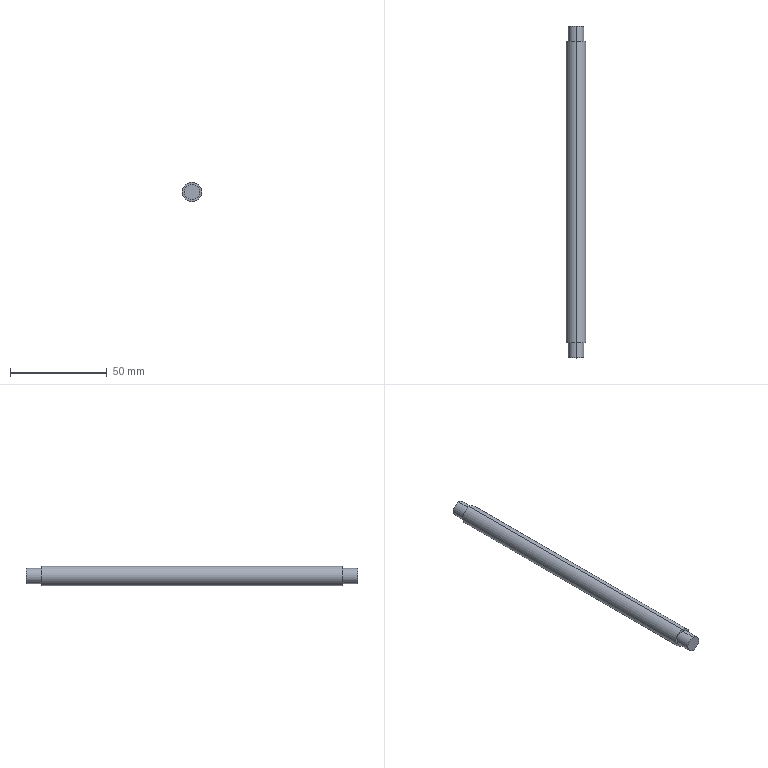Part | SolidWorks | features Extrusion 1, ICE 1, MirrorPattern 1 | 1 solid | 10 faces | box 10 x 172 x 10 mm | volume 13056 mm3 | cylinder 6 | plane 4 | commonest cylinder face diameters 8 x4 10 x2
STEP:
#1=CARTESIAN_POINT('',(0.,-3.386,0.1575));
#2=VERTEX_POINT('',#1);
#3=CARTESIAN_POINT('',(0.,-3.386,-0.1575));
#4=VERTEX_POINT('',#3);
#5=CARTESIAN_POINT('',(0.,-3.386,0.));
#6=DIRECTION('',(0.,1.,0.));
#7=DIRECTION('',(0.,0.,1.));
#8=AXIS2_PLACEMENT_3D('',#5,#6,#7);
#9=CIRCLE('',#8,0.1575);
#10=EDGE_CURVE('',#2,#4,#9,.T.);
#11=ORIENTED_EDGE('',*,*,#10,.T.);
#12=CARTESIAN_POINT('',(0.,-3.071,-0.1575));
#13=VERTEX_POINT('',#12);
#14=CARTESIAN_POINT('',(0.,-3.386,-0.1575));
#15=DIRECTION('',(0.,1.,0.));
#16=VECTOR('',#15,39.37);
#17=LINE('',#14,#16);
#18=EDGE_CURVE('',#4,#13,#17,.T.);
#19=ORIENTED_EDGE('',*,*,#18,.T.);
#20=CARTESIAN_POINT('',(0.,-3.071,0.1575));
#21=VERTEX_POINT('',#20);
#22=CARTESIAN_POINT('',(0.,-3.071,0.));
#23=DIRECTION('',(0.,1.,0.));
#24=DIRECTION('',(0.,0.,1.));
#25=AXIS2_PLACEMENT_3D('',#22,#23,#24);
#26=CIRCLE('',#25,0.1575);
#27=EDGE_CURVE('',#21,#13,#26,.T.);
#28=ORIENTED_EDGE('',*,*,#27,.F.);
#29=CARTESIAN_POINT('',(0.,-3.386,0.1575));
#30=DIRECTION('',(0.,1.,0.));
#31=VECTOR('',#30,39.37);
#32=LINE('',#29,#31);
#33=EDGE_CURVE('',#2,#21,#32,.T.);
#34=ORIENTED_EDGE('',*,*,#33,.F.);
#35=EDGE_LOOP('',(#11,#19,#28,#34));
#36=FACE_OUTER_BOUND('',#35,.T.);
#37=CARTESIAN_POINT('',(0.,-3.386,0.));
#38=DIRECTION('',(0.,1.,0.));
#39=DIRECTION('',(0.,0.,1.));
#40=AXIS2_PLACEMENT_3D('',#37,#38,#39);
#41=CYLINDRICAL_SURFACE('',#40,0.1575);
#42=ADVANCED_FACE('',(#36),#41,.T.);
#43=CARTESIAN_POINT('',(0.,3.386,0.1575));
#44=VERTEX_POINT('',#43);
#45=CARTESIAN_POINT('',(0.,3.386,-0.1575));
#46=VERTEX_POINT('',#45);
#47=CARTESIAN_POINT('',(0.,3.386,0.));
#48=DIRECTION('',(0.,1.,0.));
#49=DIRECTION('',(0.,0.,1.));
#50=AXIS2_PLACEMENT_3D('',#47,#48,#49);
#51=CIRCLE('',#50,0.1575);
#52=EDGE_CURVE('',#44,#46,#51,.T.);
#53=ORIENTED_EDGE('',*,*,#52,.F.);
#54=CARTESIAN_POINT('',(0.,3.071,0.1575));
#55=VERTEX_POINT('',#54);
#56=CARTESIAN_POINT('',(0.,3.386,0.1575));
#57=DIRECTION('',(0.,-1.,0.));
#58=VECTOR('',#57,39.37);
#59=LINE('',#56,#58);
#60=EDGE_CURVE('',#44,#55,#59,.T.);
#61=ORIENTED_EDGE('',*,*,#60,.T.);
#62=CARTESIAN_POINT('',(0.,3.071,-0.1575));
#63=VERTEX_POINT('',#62);
#64=CARTESIAN_POINT('',(0.,3.071,0.));
#65=DIRECTION('',(0.,1.,0.));
#66=DIRECTION('',(0.,0.,1.));
#67=AXIS2_PLACEMENT_3D('',#64,#65,#66);
#68=CIRCLE('',#67,0.1575);
#69=EDGE_CURVE('',#55,#63,#68,.T.);
#70=ORIENTED_EDGE('',*,*,#69,.T.);
#71=CARTESIAN_POINT('',(0.,3.386,-0.1575));
#72=DIRECTION('',(0.,-1.,0.));
#73=VECTOR('',#72,39.37);
#74=LINE('',#71,#73);
#75=EDGE_CURVE('',#46,#63,#74,.T.);
#76=ORIENTED_EDGE('',*,*,#75,.F.);
#77=EDGE_LOOP('',(#53,#61,#70,#76));
#78=FACE_OUTER_BOUND('',#77,.T.);
#79=CARTESIAN_POINT('',(0.,3.386,0.));
#80=DIRECTION('',(0.,-1.,0.));
#81=DIRECTION('',(0.,0.,-1.));
#82=AXIS2_PLACEMENT_3D('',#79,#80,#81);
#83=CYLINDRICAL_SURFACE('',#82,0.1575);
#84=ADVANCED_FACE('',(#78),#83,.T.);
#85=CARTESIAN_POINT('',(0.,3.071,0.1969));
#86=VERTEX_POINT('',#85);
#87=CARTESIAN_POINT('',(0.,3.071,-0.1969));
#88=VERTEX_POINT('',#87);
#89=CARTESIAN_POINT('',(0.,3.071,0.));
#90=DIRECTION('',(0.,1.,0.));
#91=DIRECTION('',(0.,0.,1.));
#92=AXIS2_PLACEMENT_3D('',#89,#90,#91);
#93=CIRCLE('',#92,0.1969);
#94=EDGE_CURVE('',#86,#88,#93,.T.);
#95=ORIENTED_EDGE('',*,*,#94,.F.);
#96=CARTESIAN_POINT('',(0.,-3.071,0.1969));
#97=VERTEX_POINT('',#96);
#98=CARTESIAN_POINT('',(0.,3.071,0.1969));
#99=DIRECTION('',(0.,-1.,0.));
#100=VECTOR('',#99,39.37);
#101=LINE('',#98,#100);
#102=EDGE_CURVE('',#86,#97,#101,.T.);
#103=ORIENTED_EDGE('',*,*,#102,.T.);
#104=CARTESIAN_POINT('',(0.,-3.071,-0.1969));
#105=VERTEX_POINT('',#104);
#106=CARTESIAN_POINT('',(0.,-3.071,0.));
#107=DIRECTION('',(0.,1.,0.));
#108=DIRECTION('',(0.,0.,1.));
#109=AXIS2_PLACEMENT_3D('',#106,#107,#108);
#110=CIRCLE('',#109,0.1969);
#111=EDGE_CURVE('',#97,#105,#110,.T.);
#112=ORIENTED_EDGE('',*,*,#111,.T.);
#113=CARTESIAN_POINT('',(0.,3.071,-0.1969));
#114=DIRECTION('',(0.,-1.,0.));
#115=VECTOR('',#114,39.37);
#116=LINE('',#113,#115);
#117=EDGE_CURVE('',#88,#105,#116,.T.);
#118=ORIENTED_EDGE('',*,*,#117,.F.);
#119=EDGE_LOOP('',(#95,#103,#112,#118));
#120=FACE_OUTER_BOUND('',#119,.T.);
#121=CARTESIAN_POINT('',(0.,3.071,0.));
#122=DIRECTION('',(0.,-1.,0.));
#123=DIRECTION('',(0.,0.,-1.));
#124=AXIS2_PLACEMENT_3D('',#121,#122,#123);
#125=CYLINDRICAL_SURFACE('',#124,0.1969);
#126=ADVANCED_FACE('',(#120),#125,.T.);
#127=ORIENTED_EDGE('',*,*,#102,.F.);
#128=CARTESIAN_POINT('',(0.,3.071,0.));
#129=DIRECTION('',(0.,1.,0.));
#130=DIRECTION('',(0.,0.,1.));
#131=AXIS2_PLACEMENT_3D('',#128,#129,#130);
#132=CIRCLE('',#131,0.1969);
#133=EDGE_CURVE('',#88,#86,#132,.T.);
#134=ORIENTED_EDGE('',*,*,#133,.F.);
#135=ORIENTED_EDGE('',*,*,#117,.T.);
#136=CARTESIAN_POINT('',(0.,-3.071,0.));
#137=DIRECTION('',(0.,1.,0.));
#138=DIRECTION('',(0.,0.,1.));
#139=AXIS2_PLACEMENT_3D('',#136,#137,#138);
#140=CIRCLE('',#139,0.1969);
#141=EDGE_CURVE('',#105,#97,#140,.T.);
#142=ORIENTED_EDGE('',*,*,#141,.T.);
#143=EDGE_LOOP('',(#127,#134,#135,#142));
#144=FACE_OUTER_BOUND('',#143,.T.);
#145=CARTESIAN_POINT('',(0.,3.071,0.));
#146=DIRECTION('',(0.,-1.,0.));
#147=DIRECTION('',(0.,0.,-1.));
#148=AXIS2_PLACEMENT_3D('',#145,#146,#147);
#149=CYLINDRICAL_SURFACE('',#148,0.1969);
#150=ADVANCED_FACE('',(#144),#149,.T.);
#151=CARTESIAN_POINT('',(0.,3.071,0.));
#152=DIRECTION('',(0.,1.,0.));
#153=DIRECTION('',(0.,0.,1.));
#154=AXIS2_PLACEMENT_3D('',#151,#152,#153);
#155=CIRCLE('',#154,0.1575);
#156=EDGE_CURVE('',#63,#55,#155,.T.);
#157=ORIENTED_EDGE('',*,*,#156,.F.);
#158=ORIENTED_EDGE('',*,*,#69,.F.);
#159=EDGE_LOOP('',(#157,#158));
#160=FACE_BOUND('',#159,.T.);
#161=ORIENTED_EDGE('',*,*,#133,.T.);
#162=ORIENTED_EDGE('',*,*,#94,.T.);
#163=EDGE_LOOP('',(#161,#162));
#164=FACE_OUTER_BOUND('',#163,.T.);
#165=CARTESIAN_POINT('',(0.,3.071,0.));
#166=DIRECTION('',(0.,1.,0.));
#167=DIRECTION('',(0.,0.,1.));
#168=AXIS2_PLACEMENT_3D('',#165,#166,#167);
#169=PLANE('',#168);
#170=ADVANCED_FACE('',(#160,#164),#169,.T.);
#171=ORIENTED_EDGE('',*,*,#27,.T.);
#172=CARTESIAN_POINT('',(0.,-3.071,0.));
#173=DIRECTION('',(0.,1.,0.));
#174=DIRECTION('',(0.,0.,1.));
#175=AXIS2_PLACEMENT_3D('',#172,#173,#174);
#176=CIRCLE('',#175,0.1575);
#177=EDGE_CURVE('',#13,#21,#176,.T.);
#178=ORIENTED_EDGE('',*,*,#177,.T.);
#179=EDGE_LOOP('',(#171,#178));
#180=FACE_BOUND('',#179,.T.);
#181=ORIENTED_EDGE('',*,*,#141,.F.);
#182=ORIENTED_EDGE('',*,*,#111,.F.);
#183=EDGE_LOOP('',(#181,#182));
#184=FACE_OUTER_BOUND('',#183,.T.);
#185=CARTESIAN_POINT('',(0.,-3.071,0.));
#186=DIRECTION('',(0.,1.,0.));
#187=DIRECTION('',(0.,0.,1.));
#188=AXIS2_PLACEMENT_3D('',#185,#186,#187);
#189=PLANE('',#188);
#190=ADVANCED_FACE('',(#180,#184),#189,.F.);
#191=ORIENTED_EDGE('',*,*,#60,.F.);
#192=CARTESIAN_POINT('',(0.,3.386,0.));
#193=DIRECTION('',(0.,1.,0.));
#194=DIRECTION('',(0.,0.,1.));
#195=AXIS2_PLACEMENT_3D('',#192,#193,#194);
#196=CIRCLE('',#195,0.1575);
#197=EDGE_CURVE('',#46,#44,#196,.T.);
#198=ORIENTED_EDGE('',*,*,#197,.F.);
#199=ORIENTED_EDGE('',*,*,#75,.T.);
#200=ORIENTED_EDGE('',*,*,#156,.T.);
#201=EDGE_LOOP('',(#191,#198,#199,#200));
#202=FACE_OUTER_BOUND('',#201,.T.);
#203=CARTESIAN_POINT('',(0.,3.386,0.));
#204=DIRECTION('',(0.,-1.,0.));
#205=DIRECTION('',(0.,0.,-1.));
#206=AXIS2_PLACEMENT_3D('',#203,#204,#205);
#207=CYLINDRICAL_SURFACE('',#206,0.1575);
#208=ADVANCED_FACE('',(#202),#207,.T.);
#209=ORIENTED_EDGE('',*,*,#197,.T.);
#210=ORIENTED_EDGE('',*,*,#52,.T.);
#211=EDGE_LOOP('',(#209,#210));
#212=FACE_OUTER_BOUND('',#211,.T.);
#213=CARTESIAN_POINT('',(0.,3.386,0.));
#214=DIRECTION('',(0.,1.,0.));
#215=DIRECTION('',(0.,0.,1.));
#216=AXIS2_PLACEMENT_3D('',#213,#214,#215);
#217=PLANE('',#216);
#218=ADVANCED_FACE('',(#212),#217,.T.);
#219=ORIENTED_EDGE('',*,*,#18,.F.);
#220=CARTESIAN_POINT('',(0.,-3.386,0.));
#221=DIRECTION('',(0.,1.,0.));
#222=DIRECTION('',(0.,0.,1.));
#223=AXIS2_PLACEMENT_3D('',#220,#221,#222);
#224=CIRCLE('',#223,0.1575);
#225=EDGE_CURVE('',#4,#2,#224,.T.);
#226=ORIENTED_EDGE('',*,*,#225,.T.);
#227=ORIENTED_EDGE('',*,*,#33,.T.);
#228=ORIENTED_EDGE('',*,*,#177,.F.);
#229=EDGE_LOOP('',(#219,#226,#227,#228));
#230=FACE_OUTER_BOUND('',#229,.T.);
#231=CARTESIAN_POINT('',(0.,-3.386,0.));
#232=DIRECTION('',(0.,1.,0.));
#233=DIRECTION('',(0.,0.,1.));
#234=AXIS2_PLACEMENT_3D('',#231,#232,#233);
#235=CYLINDRICAL_SURFACE('',#234,0.1575);
#236=ADVANCED_FACE('',(#230),#235,.T.);
#237=ORIENTED_EDGE('',*,*,#10,.F.);
#238=ORIENTED_EDGE('',*,*,#225,.F.);
#239=EDGE_LOOP('',(#237,#238));
#240=FACE_OUTER_BOUND('',#239,.T.);
#241=CARTESIAN_POINT('',(0.,-3.386,0.));
#242=DIRECTION('',(0.,-1.,0.));
#243=DIRECTION('',(0.,0.,1.));
#244=AXIS2_PLACEMENT_3D('',#241,#242,#243);
#245=PLANE('',#244);
#246=ADVANCED_FACE('',(#240),#245,.T.);
#247=CLOSED_SHELL('',(#42,#84,#126,#150,#170,#190,#208,#218,#236,#246));
#248=MANIFOLD_SOLID_BREP('',#247);
#249=CARTESIAN_POINT('',(0.,0.,0.));
#250=DIRECTION('',(0.,0.,1.));
#251=DIRECTION('',(1.,0.,0.));
#252=AXIS2_PLACEMENT_3D('',#249,#250,#251);
#253=(LENGTH_UNIT()NAMED_UNIT(*)SI_UNIT($,.METRE.));
#254=LENGTH_MEASURE_WITH_UNIT(LENGTH_MEASURE(0.0254),#253);
#255=DIMENSIONAL_EXPONENTS(1.,0.,0.,0.,0.,0.,0.);
#256=(CONVERSION_BASED_UNIT('INCH',#254)LENGTH_UNIT()NAMED_UNIT(#255));
#257=UNCERTAINTY_MEASURE_WITH_UNIT(LENGTH_MEASURE(0.00001),#256,'','');
#258=(NAMED_UNIT(*)PLANE_ANGLE_UNIT()SI_UNIT($,.RADIAN.));
#259=(NAMED_UNIT(*)SI_UNIT($,.STERADIAN.)SOLID_ANGLE_UNIT());
#260=(GEOMETRIC_REPRESENTATION_CONTEXT(3)GLOBAL_UNCERTAINTY_ASSIGNED_CONTEXT((#257))GLOBAL_UNIT_ASSIGNED_CONTEXT((#256,#258,#259))REPRESENTATION_CONTEXT('',''));
#261=ADVANCED_BREP_SHAPE_REPRESENTATION('',(#248,#252),#260);